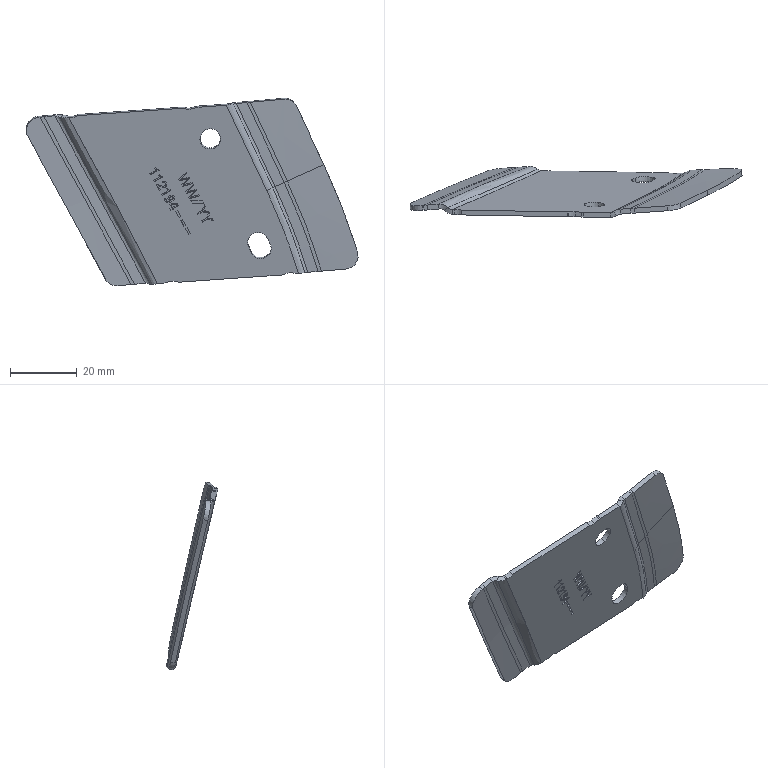Part | CATIA | 2 solids | 290 faces | box 99.513 x 15.41 x 56.212 mm | volume 6324 mm3 | plane 209 | spline 65 | cylinder 12 | other 4 | commonest cylinder face diameters 6 x6 40 x6